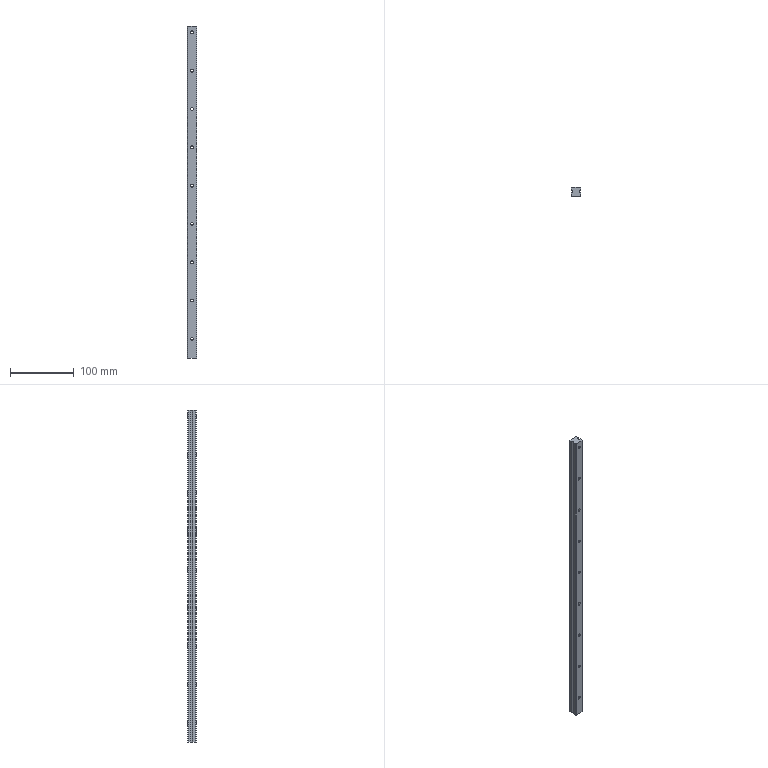Part | Creo | features CUT 12, CURVE 3, DATUM PLANE 3, COORDINATE SYSTEM 1, PATTERN 1, PROTRUSION 1 | 1 solid | 59 faces | volume 96624 mm3 | cylinder 38 | plane 21 | commonest cylinder face diameters 4.5 x18 7.5 x18 4.48 x2